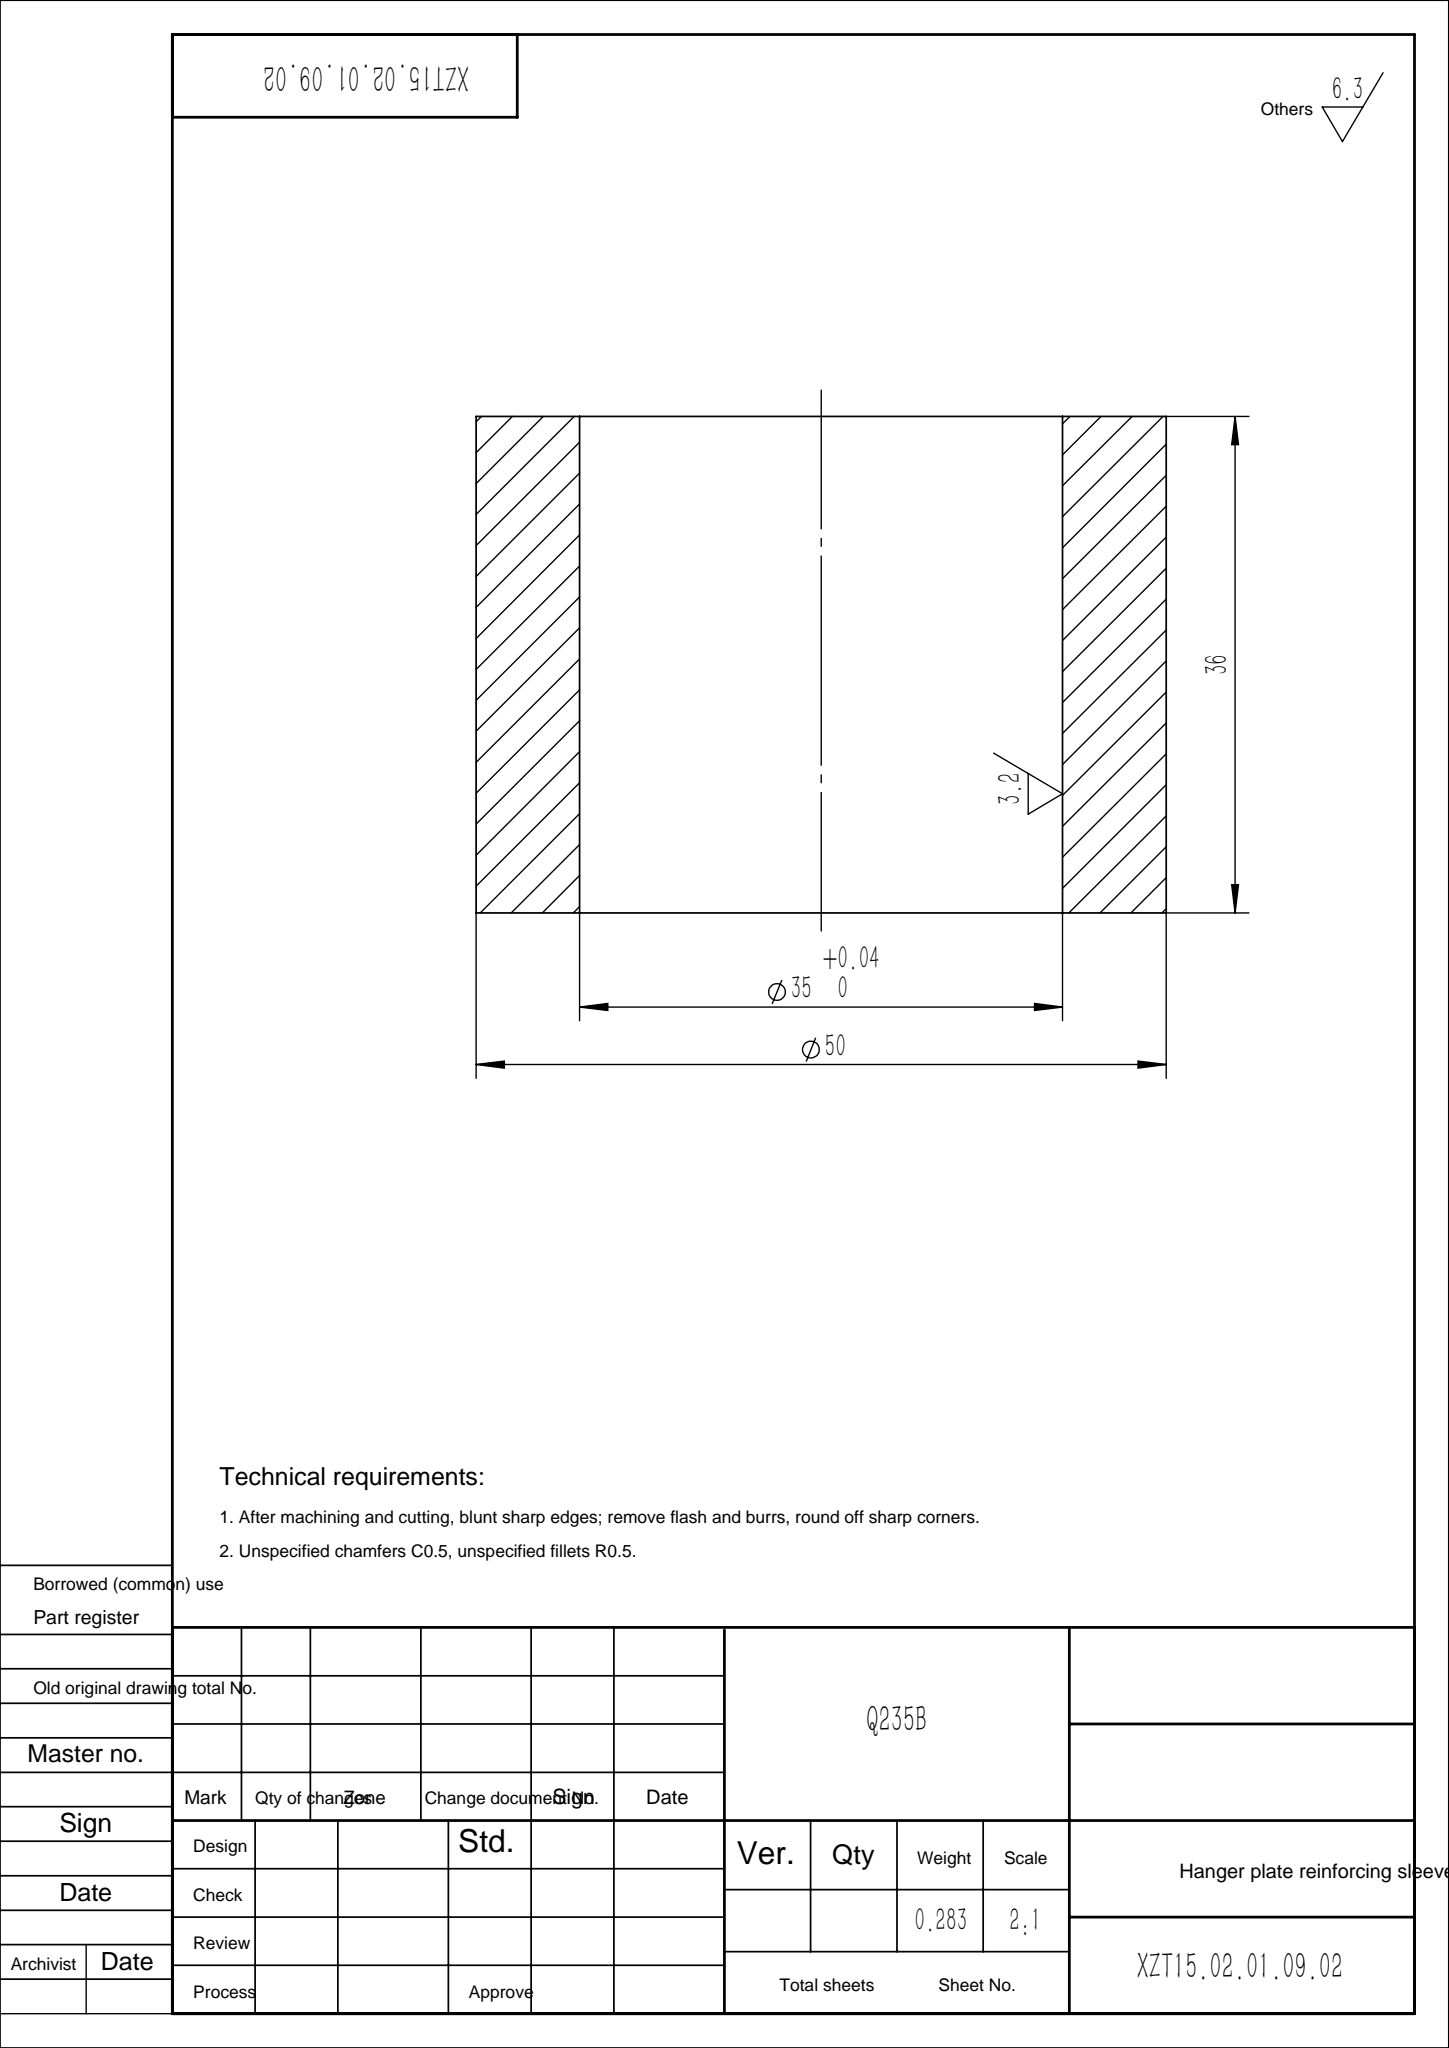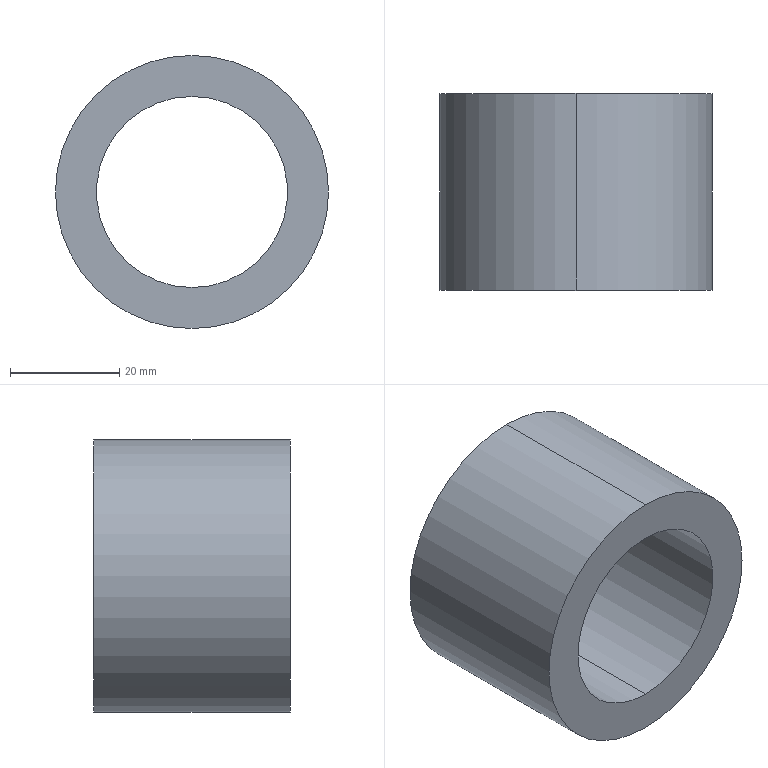Part | SolidWorks | features Extrusion 1 | 1 solid | 6 faces | box 50 x 36 x 50 mm | volume 36050 mm3 | cylinder 4 | plane 2 | commonest cylinder face diameters 35 x2 50 x2
STEP:
#1=CARTESIAN_POINT('',(0.,36.,-17.5));
#2=VERTEX_POINT('',#1);
#3=CARTESIAN_POINT('',(0.,36.,17.5));
#4=VERTEX_POINT('',#3);
#5=CARTESIAN_POINT('',(0.,36.,0.));
#6=DIRECTION('',(0.,1.,0.));
#7=DIRECTION('',(0.,0.,1.));
#8=AXIS2_PLACEMENT_3D('',#5,#6,#7);
#9=CIRCLE('',#8,17.5);
#10=EDGE_CURVE('',#2,#4,#9,.T.);
#11=ORIENTED_EDGE('',*,*,#10,.T.);
#12=CARTESIAN_POINT('',(0.,0.,17.5));
#13=VERTEX_POINT('',#12);
#14=CARTESIAN_POINT('',(0.,36.,17.5));
#15=DIRECTION('',(0.,-1.,0.));
#16=VECTOR('',#15,1000.);
#17=LINE('',#14,#16);
#18=EDGE_CURVE('',#4,#13,#17,.T.);
#19=ORIENTED_EDGE('',*,*,#18,.T.);
#20=CARTESIAN_POINT('',(0.,0.,-17.5));
#21=VERTEX_POINT('',#20);
#22=CARTESIAN_POINT('',(0.,0.,0.));
#23=DIRECTION('',(0.,1.,0.));
#24=DIRECTION('',(0.,0.,1.));
#25=AXIS2_PLACEMENT_3D('',#22,#23,#24);
#26=CIRCLE('',#25,17.5);
#27=EDGE_CURVE('',#21,#13,#26,.T.);
#28=ORIENTED_EDGE('',*,*,#27,.F.);
#29=CARTESIAN_POINT('',(0.,36.,-17.5));
#30=DIRECTION('',(0.,-1.,0.));
#31=VECTOR('',#30,1000.);
#32=LINE('',#29,#31);
#33=EDGE_CURVE('',#2,#21,#32,.T.);
#34=ORIENTED_EDGE('',*,*,#33,.F.);
#35=EDGE_LOOP('',(#11,#19,#28,#34));
#36=FACE_OUTER_BOUND('',#35,.T.);
#37=CARTESIAN_POINT('',(0.,36.,0.));
#38=DIRECTION('',(0.,-1.,0.));
#39=DIRECTION('',(0.,0.,-1.));
#40=AXIS2_PLACEMENT_3D('',#37,#38,#39);
#41=CYLINDRICAL_SURFACE('',#40,17.5);
#42=ADVANCED_FACE('',(#36),#41,.F.);
#43=CARTESIAN_POINT('',(0.,36.,25.));
#44=VERTEX_POINT('',#43);
#45=CARTESIAN_POINT('',(0.,36.,-25.));
#46=VERTEX_POINT('',#45);
#47=CARTESIAN_POINT('',(0.,36.,0.));
#48=DIRECTION('',(0.,1.,0.));
#49=DIRECTION('',(0.,0.,1.));
#50=AXIS2_PLACEMENT_3D('',#47,#48,#49);
#51=CIRCLE('',#50,25.);
#52=EDGE_CURVE('',#44,#46,#51,.T.);
#53=ORIENTED_EDGE('',*,*,#52,.F.);
#54=CARTESIAN_POINT('',(0.,0.,25.));
#55=VERTEX_POINT('',#54);
#56=CARTESIAN_POINT('',(0.,36.,25.));
#57=DIRECTION('',(0.,-1.,0.));
#58=VECTOR('',#57,1000.);
#59=LINE('',#56,#58);
#60=EDGE_CURVE('',#44,#55,#59,.T.);
#61=ORIENTED_EDGE('',*,*,#60,.T.);
#62=CARTESIAN_POINT('',(0.,0.,-25.));
#63=VERTEX_POINT('',#62);
#64=CARTESIAN_POINT('',(0.,0.,0.));
#65=DIRECTION('',(0.,1.,0.));
#66=DIRECTION('',(0.,0.,1.));
#67=AXIS2_PLACEMENT_3D('',#64,#65,#66);
#68=CIRCLE('',#67,25.);
#69=EDGE_CURVE('',#55,#63,#68,.T.);
#70=ORIENTED_EDGE('',*,*,#69,.T.);
#71=CARTESIAN_POINT('',(0.,36.,-25.));
#72=DIRECTION('',(0.,-1.,0.));
#73=VECTOR('',#72,1000.);
#74=LINE('',#71,#73);
#75=EDGE_CURVE('',#46,#63,#74,.T.);
#76=ORIENTED_EDGE('',*,*,#75,.F.);
#77=EDGE_LOOP('',(#53,#61,#70,#76));
#78=FACE_OUTER_BOUND('',#77,.T.);
#79=CARTESIAN_POINT('',(0.,36.,0.));
#80=DIRECTION('',(0.,-1.,0.));
#81=DIRECTION('',(0.,0.,-1.));
#82=AXIS2_PLACEMENT_3D('',#79,#80,#81);
#83=CYLINDRICAL_SURFACE('',#82,25.);
#84=ADVANCED_FACE('',(#78),#83,.T.);
#85=CARTESIAN_POINT('',(0.,36.,0.));
#86=DIRECTION('',(0.,1.,0.));
#87=DIRECTION('',(0.,0.,1.));
#88=AXIS2_PLACEMENT_3D('',#85,#86,#87);
#89=CIRCLE('',#88,25.);
#90=EDGE_CURVE('',#46,#44,#89,.T.);
#91=ORIENTED_EDGE('',*,*,#90,.T.);
#92=ORIENTED_EDGE('',*,*,#52,.T.);
#93=EDGE_LOOP('',(#91,#92));
#94=FACE_OUTER_BOUND('',#93,.T.);
#95=ORIENTED_EDGE('',*,*,#10,.F.);
#96=CARTESIAN_POINT('',(0.,36.,0.));
#97=DIRECTION('',(0.,1.,0.));
#98=DIRECTION('',(0.,0.,1.));
#99=AXIS2_PLACEMENT_3D('',#96,#97,#98);
#100=CIRCLE('',#99,17.5);
#101=EDGE_CURVE('',#4,#2,#100,.T.);
#102=ORIENTED_EDGE('',*,*,#101,.F.);
#103=EDGE_LOOP('',(#95,#102));
#104=FACE_BOUND('',#103,.T.);
#105=CARTESIAN_POINT('',(0.,36.,0.));
#106=DIRECTION('',(0.,1.,0.));
#107=DIRECTION('',(0.,0.,1.));
#108=AXIS2_PLACEMENT_3D('',#105,#106,#107);
#109=PLANE('',#108);
#110=ADVANCED_FACE('',(#94,#104),#109,.T.);
#111=CARTESIAN_POINT('',(0.,0.,0.));
#112=DIRECTION('',(0.,1.,0.));
#113=DIRECTION('',(0.,0.,1.));
#114=AXIS2_PLACEMENT_3D('',#111,#112,#113);
#115=CIRCLE('',#114,25.);
#116=EDGE_CURVE('',#63,#55,#115,.T.);
#117=ORIENTED_EDGE('',*,*,#116,.F.);
#118=ORIENTED_EDGE('',*,*,#69,.F.);
#119=EDGE_LOOP('',(#117,#118));
#120=FACE_OUTER_BOUND('',#119,.T.);
#121=ORIENTED_EDGE('',*,*,#27,.T.);
#122=CARTESIAN_POINT('',(0.,0.,0.));
#123=DIRECTION('',(0.,1.,0.));
#124=DIRECTION('',(0.,0.,1.));
#125=AXIS2_PLACEMENT_3D('',#122,#123,#124);
#126=CIRCLE('',#125,17.5);
#127=EDGE_CURVE('',#13,#21,#126,.T.);
#128=ORIENTED_EDGE('',*,*,#127,.T.);
#129=EDGE_LOOP('',(#121,#128));
#130=FACE_BOUND('',#129,.T.);
#131=CARTESIAN_POINT('',(0.,0.,0.));
#132=DIRECTION('',(0.,1.,0.));
#133=DIRECTION('',(0.,0.,1.));
#134=AXIS2_PLACEMENT_3D('',#131,#132,#133);
#135=PLANE('',#134);
#136=ADVANCED_FACE('',(#120,#130),#135,.F.);
#137=ORIENTED_EDGE('',*,*,#60,.F.);
#138=ORIENTED_EDGE('',*,*,#90,.F.);
#139=ORIENTED_EDGE('',*,*,#75,.T.);
#140=ORIENTED_EDGE('',*,*,#116,.T.);
#141=EDGE_LOOP('',(#137,#138,#139,#140));
#142=FACE_OUTER_BOUND('',#141,.T.);
#143=CARTESIAN_POINT('',(0.,36.,0.));
#144=DIRECTION('',(0.,-1.,0.));
#145=DIRECTION('',(0.,0.,-1.));
#146=AXIS2_PLACEMENT_3D('',#143,#144,#145);
#147=CYLINDRICAL_SURFACE('',#146,25.);
#148=ADVANCED_FACE('',(#142),#147,.T.);
#149=ORIENTED_EDGE('',*,*,#18,.F.);
#150=ORIENTED_EDGE('',*,*,#101,.T.);
#151=ORIENTED_EDGE('',*,*,#33,.T.);
#152=ORIENTED_EDGE('',*,*,#127,.F.);
#153=EDGE_LOOP('',(#149,#150,#151,#152));
#154=FACE_OUTER_BOUND('',#153,.T.);
#155=CARTESIAN_POINT('',(0.,36.,0.));
#156=DIRECTION('',(0.,-1.,0.));
#157=DIRECTION('',(0.,0.,-1.));
#158=AXIS2_PLACEMENT_3D('',#155,#156,#157);
#159=CYLINDRICAL_SURFACE('',#158,17.5);
#160=ADVANCED_FACE('',(#154),#159,.F.);
#161=CLOSED_SHELL('',(#42,#84,#110,#136,#148,#160));
#162=MANIFOLD_SOLID_BREP('',#161);
#163=CARTESIAN_POINT('',(0.,0.,0.));
#164=DIRECTION('',(0.,0.,1.));
#165=DIRECTION('',(1.,0.,0.));
#166=AXIS2_PLACEMENT_3D('',#163,#164,#165);
#167=(LENGTH_UNIT()NAMED_UNIT(*)SI_UNIT(.MILLI.,.METRE.));
#168=UNCERTAINTY_MEASURE_WITH_UNIT(LENGTH_MEASURE(0.00001),#167,'','');
#169=(NAMED_UNIT(*)PLANE_ANGLE_UNIT()SI_UNIT($,.RADIAN.));
#170=(NAMED_UNIT(*)SI_UNIT($,.STERADIAN.)SOLID_ANGLE_UNIT());
#171=(GEOMETRIC_REPRESENTATION_CONTEXT(3)GLOBAL_UNCERTAINTY_ASSIGNED_CONTEXT((#168))GLOBAL_UNIT_ASSIGNED_CONTEXT((#167,#169,#170))REPRESENTATION_CONTEXT('',''));
#172=ADVANCED_BREP_SHAPE_REPRESENTATION('',(#162,#166),#171);